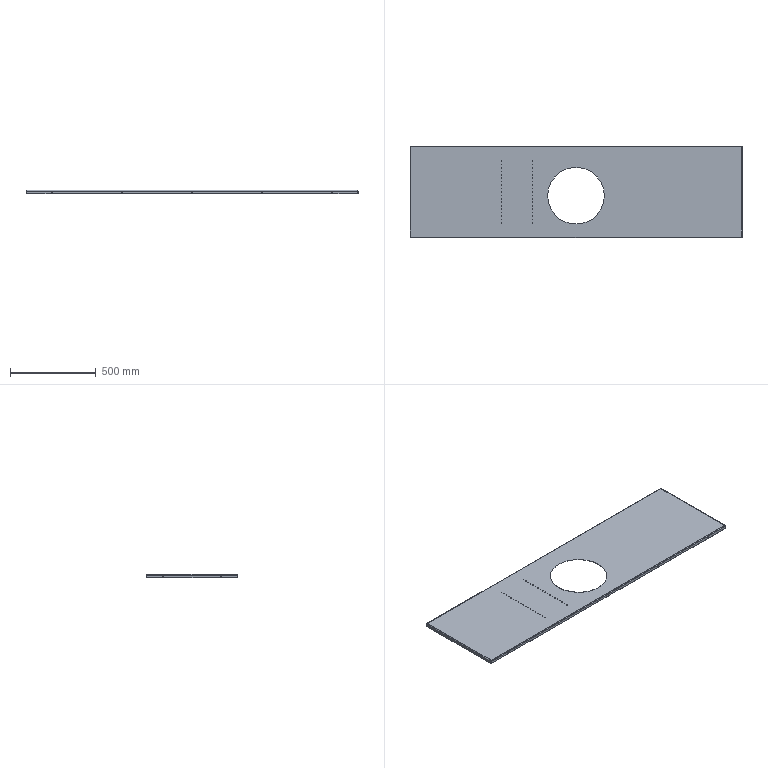Part | STEP file | JBJ-P-1011-03 | 1 solid | 133 faces | box 1935 x 535 x 20 mm | volume 1237179 mm3 | plane 64 | cylinder 61 | spline 8 | commonest cylinder face diameters 3.5 x38 6.5 x14 8 x4 10.4 x4 330 x1